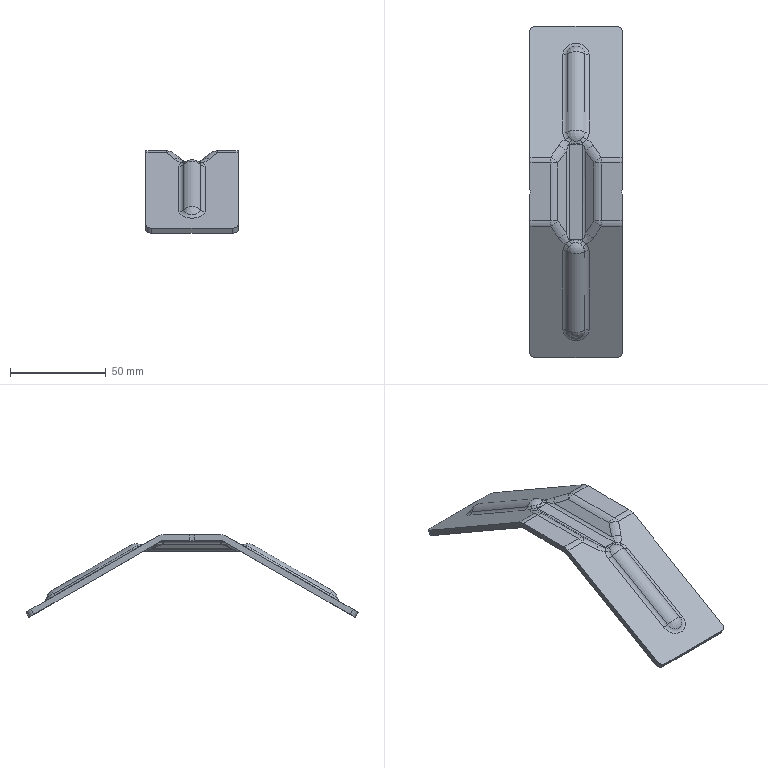Part | STEP file | 1_id210_x_t | 1 solid | 108 faces | box 48 x 173.045 x 42.999 mm | volume 28963 mm3 | cylinder 42 | spline 24 | plane 18 | sphere 12 | torus 12 | commonest cylinder face diameters 12 x12 5.85 x10 6.15 x6 12.3 x6 6 x4 9.576 x2